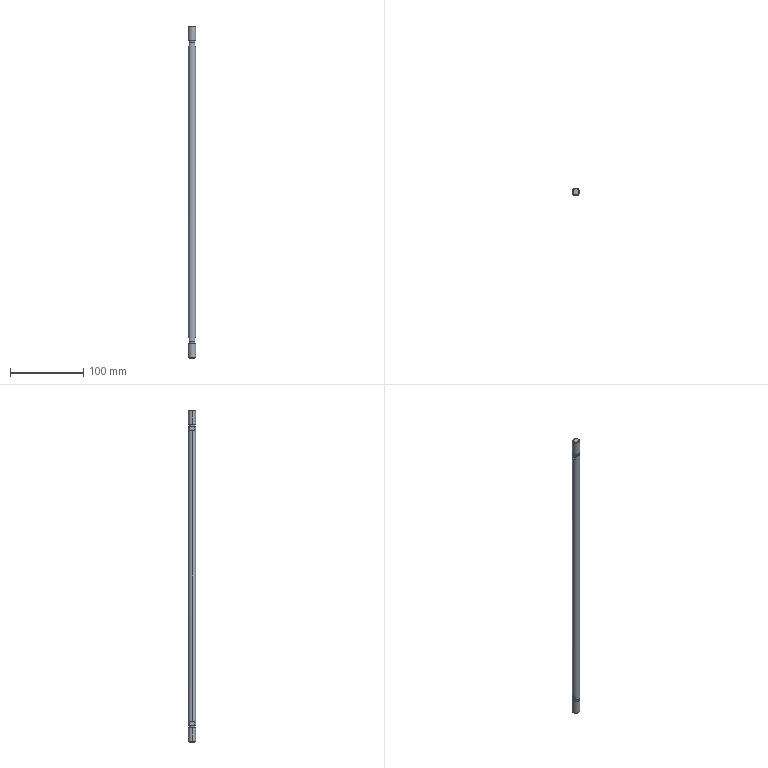Part | STEP file | rod_A_CDM2WB25_150_C76_0_ | 1 solid | 34 faces | box 10 x 10 x 452 mm | volume 35231 mm3 | plane 16 | cylinder 10 | cone 8 | commonest cylinder face diameters 10 x6 8.16 x4
STEP:
#1=CARTESIAN_POINT('',(4.08,0.,-420.));
#2=VERTEX_POINT('',#1);
#3=CARTESIAN_POINT('',(-4.08,0.,-420.));
#4=VERTEX_POINT('',#3);
#5=CARTESIAN_POINT('',(0.,0.,-420.));
#6=DIRECTION('',(0.,0.,1.));
#7=DIRECTION('',(1.,0.,0.));
#8=AXIS2_PLACEMENT_3D('',#5,#6,#7);
#9=CIRCLE('',#8,4.08);
#10=EDGE_CURVE('',#2,#4,#9,.T.);
#11=ORIENTED_EDGE('',*,*,#10,.T.);
#12=CARTESIAN_POINT('',(-5.,0.,-419.08));
#13=VERTEX_POINT('',#12);
#14=CARTESIAN_POINT('',(-4.08,0.,-420.));
#15=DIRECTION('',(-0.7071,0.,0.7071));
#16=VECTOR('',#15,1000.);
#17=LINE('',#14,#16);
#18=EDGE_CURVE('',#4,#13,#17,.T.);
#19=ORIENTED_EDGE('',*,*,#18,.T.);
#20=CARTESIAN_POINT('',(5.,0.,-419.08));
#21=VERTEX_POINT('',#20);
#22=CARTESIAN_POINT('',(0.,0.,-419.08));
#23=DIRECTION('',(0.,0.,1.));
#24=DIRECTION('',(1.,0.,0.));
#25=AXIS2_PLACEMENT_3D('',#22,#23,#24);
#26=CIRCLE('',#25,5.);
#27=EDGE_CURVE('',#21,#13,#26,.T.);
#28=ORIENTED_EDGE('',*,*,#27,.F.);
#29=CARTESIAN_POINT('',(4.08,0.,-420.));
#30=DIRECTION('',(0.7071,0.,0.7071));
#31=VECTOR('',#30,1000.);
#32=LINE('',#29,#31);
#33=EDGE_CURVE('',#2,#21,#32,.T.);
#34=ORIENTED_EDGE('',*,*,#33,.F.);
#35=EDGE_LOOP('',(#11,#19,#28,#34));
#36=FACE_OUTER_BOUND('',#35,.T.);
#37=CARTESIAN_POINT('',(0.,0.,-420.));
#38=DIRECTION('',(0.,0.,1.));
#39=DIRECTION('',(1.,0.,0.));
#40=AXIS2_PLACEMENT_3D('',#37,#38,#39);
#41=CONICAL_SURFACE('',#40,4.08,0.7854);
#42=ADVANCED_FACE('',(#36),#41,.T.);
#43=ORIENTED_EDGE('',*,*,#27,.T.);
#44=CARTESIAN_POINT('',(-5.,0.,-400.5));
#45=VERTEX_POINT('',#44);
#46=CARTESIAN_POINT('',(-5.,0.,-420.));
#47=DIRECTION('',(0.,0.,1.));
#48=VECTOR('',#47,1000.);
#49=LINE('',#46,#48);
#50=EDGE_CURVE('',#13,#45,#49,.T.);
#51=ORIENTED_EDGE('',*,*,#50,.T.);
#52=CARTESIAN_POINT('',(5.,0.,-400.5));
#53=VERTEX_POINT('',#52);
#54=CARTESIAN_POINT('',(0.,0.,-400.5));
#55=DIRECTION('',(0.,0.,1.));
#56=DIRECTION('',(1.,0.,0.));
#57=AXIS2_PLACEMENT_3D('',#54,#55,#56);
#58=CIRCLE('',#57,5.);
#59=EDGE_CURVE('',#53,#45,#58,.T.);
#60=ORIENTED_EDGE('',*,*,#59,.F.);
#61=CARTESIAN_POINT('',(5.,0.,-420.));
#62=DIRECTION('',(0.,0.,1.));
#63=VECTOR('',#62,1000.);
#64=LINE('',#61,#63);
#65=EDGE_CURVE('',#21,#53,#64,.T.);
#66=ORIENTED_EDGE('',*,*,#65,.F.);
#67=EDGE_LOOP('',(#43,#51,#60,#66));
#68=FACE_OUTER_BOUND('',#67,.T.);
#69=CARTESIAN_POINT('',(0.,0.,-420.));
#70=DIRECTION('',(0.,0.,1.));
#71=DIRECTION('',(1.,0.,0.));
#72=AXIS2_PLACEMENT_3D('',#69,#70,#71);
#73=CYLINDRICAL_SURFACE('',#72,5.);
#74=ADVANCED_FACE('',(#68),#73,.T.);
#75=CARTESIAN_POINT('',(4.08,0.,-400.5));
#76=VERTEX_POINT('',#75);
#77=CARTESIAN_POINT('',(-4.08,0.,-400.5));
#78=VERTEX_POINT('',#77);
#79=CARTESIAN_POINT('',(0.,0.,-400.5));
#80=DIRECTION('',(0.,0.,1.));
#81=DIRECTION('',(1.,0.,0.));
#82=AXIS2_PLACEMENT_3D('',#79,#80,#81);
#83=CIRCLE('',#82,4.08);
#84=EDGE_CURVE('',#76,#78,#83,.T.);
#85=ORIENTED_EDGE('',*,*,#84,.T.);
#86=CARTESIAN_POINT('',(-4.08,0.,-398.));
#87=VERTEX_POINT('',#86);
#88=CARTESIAN_POINT('',(-4.08,0.,-420.));
#89=DIRECTION('',(0.,0.,1.));
#90=VECTOR('',#89,1000.);
#91=LINE('',#88,#90);
#92=EDGE_CURVE('',#78,#87,#91,.T.);
#93=ORIENTED_EDGE('',*,*,#92,.T.);
#94=CARTESIAN_POINT('',(-4.,0.804,-398.));
#95=VERTEX_POINT('',#94);
#96=CARTESIAN_POINT('',(0.,0.,-398.));
#97=DIRECTION('',(0.,0.,1.));
#98=DIRECTION('',(1.,0.,0.));
#99=AXIS2_PLACEMENT_3D('',#96,#97,#98);
#100=CIRCLE('',#99,4.08);
#101=EDGE_CURVE('',#95,#87,#100,.T.);
#102=ORIENTED_EDGE('',*,*,#101,.F.);
#103=CARTESIAN_POINT('',(4.,0.804,-398.));
#104=VERTEX_POINT('',#103);
#105=CARTESIAN_POINT('',(0.,0.,-398.));
#106=DIRECTION('',(0.,0.,1.));
#107=DIRECTION('',(1.,0.,0.));
#108=AXIS2_PLACEMENT_3D('',#105,#106,#107);
#109=CIRCLE('',#108,4.08);
#110=EDGE_CURVE('',#104,#95,#109,.T.);
#111=ORIENTED_EDGE('',*,*,#110,.F.);
#112=CARTESIAN_POINT('',(4.08,0.,-398.));
#113=VERTEX_POINT('',#112);
#114=CARTESIAN_POINT('',(0.,0.,-398.));
#115=DIRECTION('',(0.,0.,1.));
#116=DIRECTION('',(1.,0.,0.));
#117=AXIS2_PLACEMENT_3D('',#114,#115,#116);
#118=CIRCLE('',#117,4.08);
#119=EDGE_CURVE('',#113,#104,#118,.T.);
#120=ORIENTED_EDGE('',*,*,#119,.F.);
#121=CARTESIAN_POINT('',(4.08,0.,-420.));
#122=DIRECTION('',(0.,0.,1.));
#123=VECTOR('',#122,1000.);
#124=LINE('',#121,#123);
#125=EDGE_CURVE('',#76,#113,#124,.T.);
#126=ORIENTED_EDGE('',*,*,#125,.F.);
#127=EDGE_LOOP('',(#85,#93,#102,#111,#120,#126));
#128=FACE_OUTER_BOUND('',#127,.T.);
#129=CARTESIAN_POINT('',(0.,0.,-420.));
#130=DIRECTION('',(0.,0.,1.));
#131=DIRECTION('',(1.,0.,0.));
#132=AXIS2_PLACEMENT_3D('',#129,#130,#131);
#133=CYLINDRICAL_SURFACE('',#132,4.08);
#134=ADVANCED_FACE('',(#128),#133,.T.);
#135=CARTESIAN_POINT('',(-4.,3.,-392.5));
#136=VERTEX_POINT('',#135);
#137=CARTESIAN_POINT('',(-5.,0.,-391.5));
#138=VERTEX_POINT('',#137);
#139=CARTESIAN_POINT('',(-4.,3.,-392.5));
#140=CARTESIAN_POINT('',(-4.655,2.127,-391.845));
#141=CARTESIAN_POINT('',(-5.,1.091,-391.5));
#142=CARTESIAN_POINT('',(-5.,0.,-391.5));
#143=(BOUNDED_CURVE()B_SPLINE_CURVE(3,(#139,#140,#141,#142),.UNSPECIFIED.,.F.,.T.)B_SPLINE_CURVE_WITH_KNOTS((4,4),(5.64,6.283),.UNSPECIFIED.)CURVE()GEOMETRIC_REPRESENTATION_ITEM()RATIONAL_B_SPLINE_CURVE((1.,0.9658,0.9658,1.))REPRESENTATION_ITEM(''));
#144=EDGE_CURVE('',#136,#138,#143,.T.);
#145=ORIENTED_EDGE('',*,*,#144,.T.);
#146=CARTESIAN_POINT('',(-5.,0.,3.5));
#147=VERTEX_POINT('',#146);
#148=CARTESIAN_POINT('',(-5.,0.,-420.));
#149=DIRECTION('',(0.,0.,1.));
#150=VECTOR('',#149,1000.);
#151=LINE('',#148,#150);
#152=EDGE_CURVE('',#138,#147,#151,.T.);
#153=ORIENTED_EDGE('',*,*,#152,.T.);
#154=CARTESIAN_POINT('',(-4.,3.,4.5));
#155=VERTEX_POINT('',#154);
#156=CARTESIAN_POINT('',(-5.,0.,3.5));
#157=CARTESIAN_POINT('',(-5.,1.091,3.5));
#158=CARTESIAN_POINT('',(-4.655,2.127,3.845));
#159=CARTESIAN_POINT('',(-4.,3.,4.5));
#160=(BOUNDED_CURVE()B_SPLINE_CURVE(3,(#156,#157,#158,#159),.UNSPECIFIED.,.F.,.T.)B_SPLINE_CURVE_WITH_KNOTS((4,4),(3.142,3.785),.UNSPECIFIED.)CURVE()GEOMETRIC_REPRESENTATION_ITEM()RATIONAL_B_SPLINE_CURVE((1.,0.9658,0.9658,1.))REPRESENTATION_ITEM(''));
#161=EDGE_CURVE('',#147,#155,#160,.T.);
#162=ORIENTED_EDGE('',*,*,#161,.T.);
#163=CARTESIAN_POINT('',(-4.,3.,9.08));
#164=VERTEX_POINT('',#163);
#165=CARTESIAN_POINT('',(-4.,3.,-420.));
#166=DIRECTION('',(0.,0.,1.));
#167=VECTOR('',#166,1000.);
#168=LINE('',#165,#167);
#169=EDGE_CURVE('',#155,#164,#168,.T.);
#170=ORIENTED_EDGE('',*,*,#169,.T.);
#171=CARTESIAN_POINT('',(4.,3.,9.08));
#172=VERTEX_POINT('',#171);
#173=CARTESIAN_POINT('',(0.,0.,9.08));
#174=DIRECTION('',(0.,0.,1.));
#175=DIRECTION('',(1.,0.,0.));
#176=AXIS2_PLACEMENT_3D('',#173,#174,#175);
#177=CIRCLE('',#176,5.);
#178=EDGE_CURVE('',#172,#164,#177,.T.);
#179=ORIENTED_EDGE('',*,*,#178,.F.);
#180=CARTESIAN_POINT('',(4.,3.,4.5));
#181=VERTEX_POINT('',#180);
#182=CARTESIAN_POINT('',(4.,3.,-420.));
#183=DIRECTION('',(0.,0.,-1.));
#184=VECTOR('',#183,1000.);
#185=LINE('',#182,#184);
#186=EDGE_CURVE('',#172,#181,#185,.T.);
#187=ORIENTED_EDGE('',*,*,#186,.T.);
#188=CARTESIAN_POINT('',(5.,0.,3.5));
#189=VERTEX_POINT('',#188);
#190=CARTESIAN_POINT('',(4.,3.,4.5));
#191=CARTESIAN_POINT('',(4.655,2.127,3.845));
#192=CARTESIAN_POINT('',(5.,1.091,3.5));
#193=CARTESIAN_POINT('',(5.,0.,3.5));
#194=(BOUNDED_CURVE()B_SPLINE_CURVE(3,(#190,#191,#192,#193),.UNSPECIFIED.,.F.,.T.)B_SPLINE_CURVE_WITH_KNOTS((4,4),(2.498,3.142),.UNSPECIFIED.)CURVE()GEOMETRIC_REPRESENTATION_ITEM()RATIONAL_B_SPLINE_CURVE((1.,0.9658,0.9658,1.))REPRESENTATION_ITEM(''));
#195=EDGE_CURVE('',#181,#189,#194,.T.);
#196=ORIENTED_EDGE('',*,*,#195,.T.);
#197=CARTESIAN_POINT('',(5.,0.,-391.5));
#198=VERTEX_POINT('',#197);
#199=CARTESIAN_POINT('',(5.,0.,-420.));
#200=DIRECTION('',(0.,0.,1.));
#201=VECTOR('',#200,1000.);
#202=LINE('',#199,#201);
#203=EDGE_CURVE('',#198,#189,#202,.T.);
#204=ORIENTED_EDGE('',*,*,#203,.F.);
#205=CARTESIAN_POINT('',(4.,3.,-392.5));
#206=VERTEX_POINT('',#205);
#207=CARTESIAN_POINT('',(5.,0.,-391.5));
#208=CARTESIAN_POINT('',(5.,1.091,-391.5));
#209=CARTESIAN_POINT('',(4.655,2.127,-391.845));
#210=CARTESIAN_POINT('',(4.,3.,-392.5));
#211=(BOUNDED_CURVE()B_SPLINE_CURVE(3,(#207,#208,#209,#210),.UNSPECIFIED.,.F.,.T.)B_SPLINE_CURVE_WITH_KNOTS((4,4),(0.,0.6435),.UNSPECIFIED.)CURVE()GEOMETRIC_REPRESENTATION_ITEM()RATIONAL_B_SPLINE_CURVE((1.,0.9658,0.9658,1.))REPRESENTATION_ITEM(''));
#212=EDGE_CURVE('',#198,#206,#211,.T.);
#213=ORIENTED_EDGE('',*,*,#212,.T.);
#214=CARTESIAN_POINT('',(4.,3.,-397.08));
#215=VERTEX_POINT('',#214);
#216=CARTESIAN_POINT('',(4.,3.,-420.));
#217=DIRECTION('',(0.,0.,-1.));
#218=VECTOR('',#217,1000.);
#219=LINE('',#216,#218);
#220=EDGE_CURVE('',#206,#215,#219,.T.);
#221=ORIENTED_EDGE('',*,*,#220,.T.);
#222=CARTESIAN_POINT('',(-4.,3.,-397.08));
#223=VERTEX_POINT('',#222);
#224=CARTESIAN_POINT('',(0.,0.,-397.08));
#225=DIRECTION('',(0.,0.,1.));
#226=DIRECTION('',(1.,0.,0.));
#227=AXIS2_PLACEMENT_3D('',#224,#225,#226);
#228=CIRCLE('',#227,5.);
#229=EDGE_CURVE('',#215,#223,#228,.T.);
#230=ORIENTED_EDGE('',*,*,#229,.T.);
#231=CARTESIAN_POINT('',(-4.,3.,-420.));
#232=DIRECTION('',(0.,0.,1.));
#233=VECTOR('',#232,1000.);
#234=LINE('',#231,#233);
#235=EDGE_CURVE('',#223,#136,#234,.T.);
#236=ORIENTED_EDGE('',*,*,#235,.T.);
#237=EDGE_LOOP('',(#145,#153,#162,#170,#179,#187,#196,#204,#213,#221,#230,#236));
#238=FACE_OUTER_BOUND('',#237,.T.);
#239=CARTESIAN_POINT('',(0.,0.,-420.));
#240=DIRECTION('',(0.,0.,1.));
#241=DIRECTION('',(1.,0.,0.));
#242=AXIS2_PLACEMENT_3D('',#239,#240,#241);
#243=CYLINDRICAL_SURFACE('',#242,5.);
#244=ADVANCED_FACE('',(#238),#243,.T.);
#245=CARTESIAN_POINT('',(-4.,0.804,10.));
#246=VERTEX_POINT('',#245);
#247=CARTESIAN_POINT('',(-4.08,0.,10.));
#248=VERTEX_POINT('',#247);
#249=CARTESIAN_POINT('',(0.,0.,10.));
#250=DIRECTION('',(0.,0.,1.));
#251=DIRECTION('',(1.,0.,0.));
#252=AXIS2_PLACEMENT_3D('',#249,#250,#251);
#253=CIRCLE('',#252,4.08);
#254=EDGE_CURVE('',#246,#248,#253,.T.);
#255=ORIENTED_EDGE('',*,*,#254,.T.);
#256=CARTESIAN_POINT('',(-4.08,0.,12.5));
#257=VERTEX_POINT('',#256);
#258=CARTESIAN_POINT('',(-4.08,0.,-420.));
#259=DIRECTION('',(0.,0.,1.));
#260=VECTOR('',#259,1000.);
#261=LINE('',#258,#260);
#262=EDGE_CURVE('',#248,#257,#261,.T.);
#263=ORIENTED_EDGE('',*,*,#262,.T.);
#264=CARTESIAN_POINT('',(4.08,0.,12.5));
#265=VERTEX_POINT('',#264);
#266=CARTESIAN_POINT('',(0.,0.,12.5));
#267=DIRECTION('',(0.,0.,1.));
#268=DIRECTION('',(1.,0.,0.));
#269=AXIS2_PLACEMENT_3D('',#266,#267,#268);
#270=CIRCLE('',#269,4.08);
#271=EDGE_CURVE('',#265,#257,#270,.T.);
#272=ORIENTED_EDGE('',*,*,#271,.F.);
#273=CARTESIAN_POINT('',(4.08,0.,10.));
#274=VERTEX_POINT('',#273);
#275=CARTESIAN_POINT('',(4.08,0.,-420.));
#276=DIRECTION('',(0.,0.,1.));
#277=VECTOR('',#276,1000.);
#278=LINE('',#275,#277);
#279=EDGE_CURVE('',#274,#265,#278,.T.);
#280=ORIENTED_EDGE('',*,*,#279,.F.);
#281=CARTESIAN_POINT('',(4.,0.804,10.));
#282=VERTEX_POINT('',#281);
#283=CARTESIAN_POINT('',(0.,0.,10.));
#284=DIRECTION('',(0.,0.,1.));
#285=DIRECTION('',(1.,0.,0.));
#286=AXIS2_PLACEMENT_3D('',#283,#284,#285);
#287=CIRCLE('',#286,4.08);
#288=EDGE_CURVE('',#274,#282,#287,.T.);
#289=ORIENTED_EDGE('',*,*,#288,.T.);
#290=CARTESIAN_POINT('',(0.,0.,10.));
#291=DIRECTION('',(0.,0.,1.));
#292=DIRECTION('',(1.,0.,0.));
#293=AXIS2_PLACEMENT_3D('',#290,#291,#292);
#294=CIRCLE('',#293,4.08);
#295=EDGE_CURVE('',#282,#246,#294,.T.);
#296=ORIENTED_EDGE('',*,*,#295,.T.);
#297=EDGE_LOOP('',(#255,#263,#272,#280,#289,#296));
#298=FACE_OUTER_BOUND('',#297,.T.);
#299=CARTESIAN_POINT('',(0.,0.,-420.));
#300=DIRECTION('',(0.,0.,1.));
#301=DIRECTION('',(1.,0.,0.));
#302=AXIS2_PLACEMENT_3D('',#299,#300,#301);
#303=CYLINDRICAL_SURFACE('',#302,4.08);
#304=ADVANCED_FACE('',(#298),#303,.T.);
#305=CARTESIAN_POINT('',(5.,0.,12.5));
#306=VERTEX_POINT('',#305);
#307=CARTESIAN_POINT('',(-5.,0.,12.5));
#308=VERTEX_POINT('',#307);
#309=CARTESIAN_POINT('',(0.,0.,12.5));
#310=DIRECTION('',(0.,0.,1.));
#311=DIRECTION('',(1.,0.,0.));
#312=AXIS2_PLACEMENT_3D('',#309,#310,#311);
#313=CIRCLE('',#312,5.);
#314=EDGE_CURVE('',#306,#308,#313,.T.);
#315=ORIENTED_EDGE('',*,*,#314,.T.);
#316=CARTESIAN_POINT('',(-5.,0.,31.08));
#317=VERTEX_POINT('',#316);
#318=CARTESIAN_POINT('',(-5.,0.,-420.));
#319=DIRECTION('',(0.,0.,1.));
#320=VECTOR('',#319,1000.);
#321=LINE('',#318,#320);
#322=EDGE_CURVE('',#308,#317,#321,.T.);
#323=ORIENTED_EDGE('',*,*,#322,.T.);
#324=CARTESIAN_POINT('',(5.,0.,31.08));
#325=VERTEX_POINT('',#324);
#326=CARTESIAN_POINT('',(0.,0.,31.08));
#327=DIRECTION('',(0.,0.,1.));
#328=DIRECTION('',(1.,0.,0.));
#329=AXIS2_PLACEMENT_3D('',#326,#327,#328);
#330=CIRCLE('',#329,5.);
#331=EDGE_CURVE('',#325,#317,#330,.T.);
#332=ORIENTED_EDGE('',*,*,#331,.F.);
#333=CARTESIAN_POINT('',(5.,0.,-420.));
#334=DIRECTION('',(0.,0.,1.));
#335=VECTOR('',#334,1000.);
#336=LINE('',#333,#335);
#337=EDGE_CURVE('',#306,#325,#336,.T.);
#338=ORIENTED_EDGE('',*,*,#337,.F.);
#339=EDGE_LOOP('',(#315,#323,#332,#338));
#340=FACE_OUTER_BOUND('',#339,.T.);
#341=CARTESIAN_POINT('',(0.,0.,-420.));
#342=DIRECTION('',(0.,0.,1.));
#343=DIRECTION('',(1.,0.,0.));
#344=AXIS2_PLACEMENT_3D('',#341,#342,#343);
#345=CYLINDRICAL_SURFACE('',#344,5.);
#346=ADVANCED_FACE('',(#340),#345,.T.);
#347=CARTESIAN_POINT('',(4.08,0.,32.));
#348=VERTEX_POINT('',#347);
#349=CARTESIAN_POINT('',(-4.08,0.,32.));
#350=VERTEX_POINT('',#349);
#351=CARTESIAN_POINT('',(0.,0.,32.));
#352=DIRECTION('',(0.,0.,1.));
#353=DIRECTION('',(1.,0.,0.));
#354=AXIS2_PLACEMENT_3D('',#351,#352,#353);
#355=CIRCLE('',#354,4.08);
#356=EDGE_CURVE('',#348,#350,#355,.T.);
#357=ORIENTED_EDGE('',*,*,#356,.F.);
#358=CARTESIAN_POINT('',(5.,0.,31.08));
#359=DIRECTION('',(0.7071,0.,-0.7071));
#360=VECTOR('',#359,1000.);
#361=LINE('',#358,#360);
#362=EDGE_CURVE('',#348,#325,#361,.T.);
#363=ORIENTED_EDGE('',*,*,#362,.T.);
#364=ORIENTED_EDGE('',*,*,#331,.T.);
#365=CARTESIAN_POINT('',(-5.,0.,31.08));
#366=DIRECTION('',(-0.7071,0.,-0.7071));
#367=VECTOR('',#366,1000.);
#368=LINE('',#365,#367);
#369=EDGE_CURVE('',#350,#317,#368,.T.);
#370=ORIENTED_EDGE('',*,*,#369,.F.);
#371=EDGE_LOOP('',(#357,#363,#364,#370));
#372=FACE_OUTER_BOUND('',#371,.T.);
#373=CARTESIAN_POINT('',(0.,0.,31.08));
#374=DIRECTION('',(0.,0.,-1.));
#375=DIRECTION('',(-1.,0.,0.));
#376=AXIS2_PLACEMENT_3D('',#373,#374,#375);
#377=CONICAL_SURFACE('',#376,5.,0.7854);
#378=ADVANCED_FACE('',(#372),#377,.T.);
#379=CARTESIAN_POINT('',(-4.,-3.,-397.08));
#380=VERTEX_POINT('',#379);
#381=CARTESIAN_POINT('',(4.,-3.,-397.08));
#382=VERTEX_POINT('',#381);
#383=CARTESIAN_POINT('',(0.,0.,-397.08));
#384=DIRECTION('',(0.,0.,1.));
#385=DIRECTION('',(1.,0.,0.));
#386=AXIS2_PLACEMENT_3D('',#383,#384,#385);
#387=CIRCLE('',#386,5.);
#388=EDGE_CURVE('',#380,#382,#387,.T.);
#389=ORIENTED_EDGE('',*,*,#388,.F.);
#390=CARTESIAN_POINT('',(-4.,-0.804,-398.));
#391=VERTEX_POINT('',#390);
#392=CARTESIAN_POINT('',(-4.,-3.,-397.08));
#393=CARTESIAN_POINT('',(-4.,-2.657,-397.286));
#394=CARTESIAN_POINT('',(-4.,-2.306,-397.474));
#395=CARTESIAN_POINT('',(-4.,-1.576,-397.793));
#396=CARTESIAN_POINT('',(-4.,-1.193,-397.923));
#397=CARTESIAN_POINT('',(-4.,-0.804,-398.));
#398=B_SPLINE_CURVE_WITH_KNOTS('',3,(#392,#393,#394,#395,#396,#397),.UNSPECIFIED.,.F.,.F.,(4,2,4),(0.00946,0.01066,0.01185),.UNSPECIFIED.);
#399=EDGE_CURVE('',#380,#391,#398,.T.);
#400=ORIENTED_EDGE('',*,*,#399,.T.);
#401=CARTESIAN_POINT('',(4.,-0.804,-398.));
#402=VERTEX_POINT('',#401);
#403=CARTESIAN_POINT('',(0.,0.,-398.));
#404=DIRECTION('',(0.,0.,1.));
#405=DIRECTION('',(1.,0.,0.));
#406=AXIS2_PLACEMENT_3D('',#403,#404,#405);
#407=CIRCLE('',#406,4.08);
#408=EDGE_CURVE('',#391,#402,#407,.T.);
#409=ORIENTED_EDGE('',*,*,#408,.T.);
#410=CARTESIAN_POINT('',(4.,-0.804,-398.));
#411=CARTESIAN_POINT('',(4.,-1.195,-397.923));
#412=CARTESIAN_POINT('',(4.,-1.58,-397.792));
#413=CARTESIAN_POINT('',(4.,-2.311,-397.472));
#414=CARTESIAN_POINT('',(4.,-2.66,-397.284));
#415=CARTESIAN_POINT('',(4.,-3.,-397.08));
#416=B_SPLINE_CURVE_WITH_KNOTS('',3,(#410,#411,#412,#413,#414,#415),.UNSPECIFIED.,.F.,.F.,(4,2,4),(0.01347,0.01467,0.01588),.UNSPECIFIED.);
#417=EDGE_CURVE('',#402,#382,#416,.T.);
#418=ORIENTED_EDGE('',*,*,#417,.T.);
#419=EDGE_LOOP('',(#389,#400,#409,#418));
#420=FACE_OUTER_BOUND('',#419,.T.);
#421=CARTESIAN_POINT('',(0.,0.,-398.));
#422=DIRECTION('',(0.,0.,1.));
#423=DIRECTION('',(1.,0.,0.));
#424=AXIS2_PLACEMENT_3D('',#421,#422,#423);
#425=CONICAL_SURFACE('',#424,4.08,0.7854);
#426=ADVANCED_FACE('',(#420),#425,.T.);
#427=ORIENTED_EDGE('',*,*,#178,.T.);
#428=CARTESIAN_POINT('',(-4.,3.,9.08));
#429=CARTESIAN_POINT('',(-4.,2.657,9.286));
#430=CARTESIAN_POINT('',(-4.,2.306,9.474));
#431=CARTESIAN_POINT('',(-4.,1.576,9.793));
#432=CARTESIAN_POINT('',(-4.,1.193,9.923));
#433=CARTESIAN_POINT('',(-4.,0.804,10.));
#434=B_SPLINE_CURVE_WITH_KNOTS('',3,(#428,#429,#430,#431,#432,#433),.UNSPECIFIED.,.F.,.F.,(4,2,4),(0.00946,0.01066,0.01185),.UNSPECIFIED.);
#435=EDGE_CURVE('',#164,#246,#434,.T.);
#436=ORIENTED_EDGE('',*,*,#435,.T.);
#437=ORIENTED_EDGE('',*,*,#295,.F.);
#438=CARTESIAN_POINT('',(4.,0.804,10.));
#439=CARTESIAN_POINT('',(4.,1.195,9.923));
#440=CARTESIAN_POINT('',(4.,1.58,9.792));
#441=CARTESIAN_POINT('',(4.,2.311,9.472));
#442=CARTESIAN_POINT('',(4.,2.66,9.284));
#443=CARTESIAN_POINT('',(4.,3.,9.08));
#444=B_SPLINE_CURVE_WITH_KNOTS('',3,(#438,#439,#440,#441,#442,#443),.UNSPECIFIED.,.F.,.F.,(4,2,4),(0.01347,0.01467,0.01588),.UNSPECIFIED.);
#445=EDGE_CURVE('',#282,#172,#444,.T.);
#446=ORIENTED_EDGE('',*,*,#445,.T.);
#447=EDGE_LOOP('',(#427,#436,#437,#446));
#448=FACE_OUTER_BOUND('',#447,.T.);
#449=CARTESIAN_POINT('',(0.,0.,9.08));
#450=DIRECTION('',(0.,0.,-1.));
#451=DIRECTION('',(-1.,0.,0.));
#452=AXIS2_PLACEMENT_3D('',#449,#450,#451);
#453=CONICAL_SURFACE('',#452,5.,0.7854);
#454=ADVANCED_FACE('',(#448),#453,.T.);
#455=CARTESIAN_POINT('',(0.,0.,32.));
#456=DIRECTION('',(0.,0.,1.));
#457=DIRECTION('',(1.,0.,0.));
#458=AXIS2_PLACEMENT_3D('',#455,#456,#457);
#459=CIRCLE('',#458,4.08);
#460=EDGE_CURVE('',#350,#348,#459,.T.);
#461=ORIENTED_EDGE('',*,*,#460,.T.);
#462=ORIENTED_EDGE('',*,*,#356,.T.);
#463=EDGE_LOOP('',(#461,#462));
#464=FACE_OUTER_BOUND('',#463,.T.);
#465=CARTESIAN_POINT('',(0.,0.,32.));
#466=DIRECTION('',(0.,0.,-1.));
#467=DIRECTION('',(-1.,0.,0.));
#468=AXIS2_PLACEMENT_3D('',#465,#466,#467);
#469=PLANE('',#468);
#470=ADVANCED_FACE('',(#464),#469,.F.);
#471=ORIENTED_EDGE('',*,*,#362,.F.);
#472=ORIENTED_EDGE('',*,*,#460,.F.);
#473=ORIENTED_EDGE('',*,*,#369,.T.);
#474=CARTESIAN_POINT('',(0.,0.,31.08));
#475=DIRECTION('',(0.,0.,1.));
#476=DIRECTION('',(1.,0.,0.));
#477=AXIS2_PLACEMENT_3D('',#474,#475,#476);
#478=CIRCLE('',#477,5.);
#479=EDGE_CURVE('',#317,#325,#478,.T.);
#480=ORIENTED_EDGE('',*,*,#479,.T.);
#481=EDGE_LOOP('',(#471,#472,#473,#480));
#482=FACE_OUTER_BOUND('',#481,.T.);
#483=CARTESIAN_POINT('',(0.,0.,31.08));
#484=DIRECTION('',(0.,0.,-1.));
#485=DIRECTION('',(-1.,0.,0.));
#486=AXIS2_PLACEMENT_3D('',#483,#484,#485);
#487=CONICAL_SURFACE('',#486,5.,0.7854);
#488=ADVANCED_FACE('',(#482),#487,.T.);
#489=ORIENTED_EDGE('',*,*,#322,.F.);
#490=CARTESIAN_POINT('',(0.,0.,12.5));
#491=DIRECTION('',(0.,0.,1.));
#492=DIRECTION('',(1.,0.,0.));
#493=AXIS2_PLACEMENT_3D('',#490,#491,#492);
#494=CIRCLE('',#493,5.);
#495=EDGE_CURVE('',#308,#306,#494,.T.);
#496=ORIENTED_EDGE('',*,*,#495,.T.);
#497=ORIENTED_EDGE('',*,*,#337,.T.);
#498=ORIENTED_EDGE('',*,*,#479,.F.);
#499=EDGE_LOOP('',(#489,#496,#497,#498));
#500=FACE_OUTER_BOUND('',#499,.T.);
#501=CARTESIAN_POINT('',(0.,0.,-420.));
#502=DIRECTION('',(0.,0.,1.));
#503=DIRECTION('',(1.,0.,0.));
#504=AXIS2_PLACEMENT_3D('',#501,#502,#503);
#505=CYLINDRICAL_SURFACE('',#504,5.);
#506=ADVANCED_FACE('',(#500),#505,.T.);
#507=ORIENTED_EDGE('',*,*,#314,.F.);
#508=ORIENTED_EDGE('',*,*,#495,.F.);
#509=EDGE_LOOP('',(#507,#508));
#510=FACE_OUTER_BOUND('',#509,.T.);
#511=ORIENTED_EDGE('',*,*,#271,.T.);
#512=CARTESIAN_POINT('',(0.,0.,12.5));
#513=DIRECTION('',(0.,0.,1.));
#514=DIRECTION('',(1.,0.,0.));
#515=AXIS2_PLACEMENT_3D('',#512,#513,#514);
#516=CIRCLE('',#515,4.08);
#517=EDGE_CURVE('',#257,#265,#516,.T.);
#518=ORIENTED_EDGE('',*,*,#517,.T.);
#519=EDGE_LOOP('',(#511,#518));
#520=FACE_BOUND('',#519,.T.);
#521=CARTESIAN_POINT('',(0.,5.,12.5));
#522=DIRECTION('',(0.,0.,1.));
#523=DIRECTION('',(1.,0.,0.));
#524=AXIS2_PLACEMENT_3D('',#521,#522,#523);
#525=PLANE('',#524);
#526=ADVANCED_FACE('',(#510,#520),#525,.F.);
#527=ORIENTED_EDGE('',*,*,#262,.F.);
#528=CARTESIAN_POINT('',(-4.,-0.804,10.));
#529=VERTEX_POINT('',#528);
#530=CARTESIAN_POINT('',(0.,0.,10.));
#531=DIRECTION('',(0.,0.,1.));
#532=DIRECTION('',(1.,0.,0.));
#533=AXIS2_PLACEMENT_3D('',#530,#531,#532);
#534=CIRCLE('',#533,4.08);
#535=EDGE_CURVE('',#248,#529,#534,.T.);
#536=ORIENTED_EDGE('',*,*,#535,.T.);
#537=CARTESIAN_POINT('',(4.,-0.804,10.));
#538=VERTEX_POINT('',#537);
#539=CARTESIAN_POINT('',(0.,0.,10.));
#540=DIRECTION('',(0.,0.,1.));
#541=DIRECTION('',(1.,0.,0.));
#542=AXIS2_PLACEMENT_3D('',#539,#540,#541);
#543=CIRCLE('',#542,4.08);
#544=EDGE_CURVE('',#529,#538,#543,.T.);
#545=ORIENTED_EDGE('',*,*,#544,.T.);
#546=CARTESIAN_POINT('',(0.,0.,10.));
#547=DIRECTION('',(0.,0.,1.));
#548=DIRECTION('',(1.,0.,0.));
#549=AXIS2_PLACEMENT_3D('',#546,#547,#548);
#550=CIRCLE('',#549,4.08);
#551=EDGE_CURVE('',#538,#274,#550,.T.);
#552=ORIENTED_EDGE('',*,*,#551,.T.);
#553=ORIENTED_EDGE('',*,*,#279,.T.);
#554=ORIENTED_EDGE('',*,*,#517,.F.);
#555=EDGE_LOOP('',(#527,#536,#545,#552,#553,#554));
#556=FACE_OUTER_BOUND('',#555,.T.);
#557=CARTESIAN_POINT('',(0.,0.,-420.));
#558=DIRECTION('',(0.,0.,1.));
#559=DIRECTION('',(1.,0.,0.));
#560=AXIS2_PLACEMENT_3D('',#557,#558,#559);
#561=CYLINDRICAL_SURFACE('',#560,4.08);
#562=ADVANCED_FACE('',(#556),#561,.T.);
#563=ORIENTED_EDGE('',*,*,#544,.F.);
#564=CARTESIAN_POINT('',(-4.,-3.,9.08));
#565=VERTEX_POINT('',#564);
#566=CARTESIAN_POINT('',(-4.,-0.804,10.));
#567=CARTESIAN_POINT('',(-4.,-1.195,9.923));
#568=CARTESIAN_POINT('',(-4.,-1.58,9.792));
#569=CARTESIAN_POINT('',(-4.,-2.311,9.472));
#570=CARTESIAN_POINT('',(-4.,-2.66,9.284));
#571=CARTESIAN_POINT('',(-4.,-3.,9.08));
#572=B_SPLINE_CURVE_WITH_KNOTS('',3,(#566,#567,#568,#569,#570,#571),.UNSPECIFIED.,.F.,.F.,(4,2,4),(0.01347,0.01467,0.01588),.UNSPECIFIED.);
#573=EDGE_CURVE('',#529,#565,#572,.T.);
#574=ORIENTED_EDGE('',*,*,#573,.T.);
#575=CARTESIAN_POINT('',(4.,-3.,9.08));
#576=VERTEX_POINT('',#575);
#577=CARTESIAN_POINT('',(0.,0.,9.08));
#578=DIRECTION('',(0.,0.,1.));
#579=DIRECTION('',(1.,0.,0.));
#580=AXIS2_PLACEMENT_3D('',#577,#578,#579);
#581=CIRCLE('',#580,5.);
#582=EDGE_CURVE('',#565,#576,#581,.T.);
#583=ORIENTED_EDGE('',*,*,#582,.T.);
#584=CARTESIAN_POINT('',(4.,-3.,9.08));
#585=CARTESIAN_POINT('',(4.,-2.657,9.286));
#586=CARTESIAN_POINT('',(4.,-2.306,9.474));
#587=CARTESIAN_POINT('',(4.,-1.576,9.793));
#588=CARTESIAN_POINT('',(4.,-1.193,9.923));
#589=CARTESIAN_POINT('',(4.,-0.804,10.));
#590=B_SPLINE_CURVE_WITH_KNOTS('',3,(#584,#585,#586,#587,#588,#589),.UNSPECIFIED.,.F.,.F.,(4,2,4),(0.00946,0.01066,0.01185),.UNSPECIFIED.);
#591=EDGE_CURVE('',#576,#538,#590,.T.);
#592=ORIENTED_EDGE('',*,*,#591,.T.);
#593=EDGE_LOOP('',(#563,#574,#583,#592));
#594=FACE_OUTER_BOUND('',#593,.T.);
#595=CARTESIAN_POINT('',(0.,0.,9.08));
#596=DIRECTION('',(0.,0.,-1.));
#597=DIRECTION('',(-1.,0.,0.));
#598=AXIS2_PLACEMENT_3D('',#595,#596,#597);
#599=CONICAL_SURFACE('',#598,5.,0.7854);
#600=ADVANCED_FACE('',(#594),#599,.T.);
#601=ORIENTED_EDGE('',*,*,#152,.F.);
#602=CARTESIAN_POINT('',(-4.,-3.,-392.5));
#603=VERTEX_POINT('',#602);
#604=CARTESIAN_POINT('',(-5.,0.,-391.5));
#605=CARTESIAN_POINT('',(-5.,-1.091,-391.5));
#606=CARTESIAN_POINT('',(-4.655,-2.127,-391.845));
#607=CARTESIAN_POINT('',(-4.,-3.,-392.5));
#608=(BOUNDED_CURVE()B_SPLINE_CURVE(3,(#604,#605,#606,#607),.UNSPECIFIED.,.F.,.F.)B_SPLINE_CURVE_WITH_KNOTS((4,4),(0.,0.6435),.UNSPECIFIED.)CURVE()GEOMETRIC_REPRESENTATION_ITEM()RATIONAL_B_SPLINE_CURVE((1.,0.9658,0.9658,1.))REPRESENTATION_ITEM(''));
#609=EDGE_CURVE('',#138,#603,#608,.T.);
#610=ORIENTED_EDGE('',*,*,#609,.T.);
#611=CARTESIAN_POINT('',(-4.,-3.,-420.));
#612=DIRECTION('',(0.,0.,-1.));
#613=VECTOR('',#612,1000.);
#614=LINE('',#611,#613);
#615=EDGE_CURVE('',#603,#380,#614,.T.);
#616=ORIENTED_EDGE('',*,*,#615,.T.);
#617=ORIENTED_EDGE('',*,*,#388,.T.);
#618=CARTESIAN_POINT('',(4.,-3.,-392.5));
#619=VERTEX_POINT('',#618);
#620=CARTESIAN_POINT('',(4.,-3.,-420.));
#621=DIRECTION('',(0.,0.,1.));
#622=VECTOR('',#621,1000.);
#623=LINE('',#620,#622);
#624=EDGE_CURVE('',#382,#619,#623,.T.);
#625=ORIENTED_EDGE('',*,*,#624,.T.);
#626=CARTESIAN_POINT('',(4.,-3.,-392.5));
#627=CARTESIAN_POINT('',(4.655,-2.127,-391.845));
#628=CARTESIAN_POINT('',(5.,-1.091,-391.5));
#629=CARTESIAN_POINT('',(5.,0.,-391.5));
#630=(BOUNDED_CURVE()B_SPLINE_CURVE(3,(#626,#627,#628,#629),.UNSPECIFIED.,.F.,.F.)B_SPLINE_CURVE_WITH_KNOTS((4,4),(5.64,6.283),.UNSPECIFIED.)CURVE()GEOMETRIC_REPRESENTATION_ITEM()RATIONAL_B_SPLINE_CURVE((1.,0.9658,0.9658,1.))REPRESENTATION_ITEM(''));
#631=EDGE_CURVE('',#619,#198,#630,.T.);
#632=ORIENTED_EDGE('',*,*,#631,.T.);
#633=ORIENTED_EDGE('',*,*,#203,.T.);
#634=CARTESIAN_POINT('',(4.,-3.,4.5));
#635=VERTEX_POINT('',#634);
#636=CARTESIAN_POINT('',(5.,0.,3.5));
#637=CARTESIAN_POINT('',(5.,-1.091,3.5));
#638=CARTESIAN_POINT('',(4.655,-2.127,3.845));
#639=CARTESIAN_POINT('',(4.,-3.,4.5));
#640=(BOUNDED_CURVE()B_SPLINE_CURVE(3,(#636,#637,#638,#639),.UNSPECIFIED.,.F.,.F.)B_SPLINE_CURVE_WITH_KNOTS((4,4),(3.142,3.785),.UNSPECIFIED.)CURVE()GEOMETRIC_REPRESENTATION_ITEM()RATIONAL_B_SPLINE_CURVE((1.,0.9658,0.9658,1.))REPRESENTATION_ITEM(''));
#641=EDGE_CURVE('',#189,#635,#640,.T.);
#642=ORIENTED_EDGE('',*,*,#641,.T.);
#643=CARTESIAN_POINT('',(4.,-3.,-420.));
#644=DIRECTION('',(0.,0.,1.));
#645=VECTOR('',#644,1000.);
#646=LINE('',#643,#645);
#647=EDGE_CURVE('',#635,#576,#646,.T.);
#648=ORIENTED_EDGE('',*,*,#647,.T.);
#649=ORIENTED_EDGE('',*,*,#582,.F.);
#650=CARTESIAN_POINT('',(-4.,-3.,4.5));
#651=VERTEX_POINT('',#650);
#652=CARTESIAN_POINT('',(-4.,-3.,-420.));
#653=DIRECTION('',(0.,0.,-1.));
#654=VECTOR('',#653,1000.);
#655=LINE('',#652,#654);
#656=EDGE_CURVE('',#565,#651,#655,.T.);
#657=ORIENTED_EDGE('',*,*,#656,.T.);
#658=CARTESIAN_POINT('',(-4.,-3.,4.5));
#659=CARTESIAN_POINT('',(-4.655,-2.127,3.845));
#660=CARTESIAN_POINT('',(-5.,-1.091,3.5));
#661=CARTESIAN_POINT('',(-5.,0.,3.5));
#662=(BOUNDED_CURVE()B_SPLINE_CURVE(3,(#658,#659,#660,#661),.UNSPECIFIED.,.F.,.F.)B_SPLINE_CURVE_WITH_KNOTS((4,4),(2.498,3.142),.UNSPECIFIED.)CURVE()GEOMETRIC_REPRESENTATION_ITEM()RATIONAL_B_SPLINE_CURVE((1.,0.9658,0.9658,1.))REPRESENTATION_ITEM(''));
#663=EDGE_CURVE('',#651,#147,#662,.T.);
#664=ORIENTED_EDGE('',*,*,#663,.T.);
#665=EDGE_LOOP('',(#601,#610,#616,#617,#625,#632,#633,#642,#648,#649,#657,#664));
#666=FACE_OUTER_BOUND('',#665,.T.);
#667=CARTESIAN_POINT('',(0.,0.,-420.));
#668=DIRECTION('',(0.,0.,1.));
#669=DIRECTION('',(1.,0.,0.));
#670=AXIS2_PLACEMENT_3D('',#667,#668,#669);
#671=CYLINDRICAL_SURFACE('',#670,5.);
#672=ADVANCED_FACE('',(#666),#671,.T.);
#673=ORIENTED_EDGE('',*,*,#110,.T.);
#674=CARTESIAN_POINT('',(-4.,0.804,-398.));
#675=CARTESIAN_POINT('',(-4.,1.195,-397.923));
#676=CARTESIAN_POINT('',(-4.,1.58,-397.792));
#677=CARTESIAN_POINT('',(-4.,2.311,-397.472));
#678=CARTESIAN_POINT('',(-4.,2.66,-397.284));
#679=CARTESIAN_POINT('',(-4.,3.,-397.08));
#680=B_SPLINE_CURVE_WITH_KNOTS('',3,(#674,#675,#676,#677,#678,#679),.UNSPECIFIED.,.F.,.F.,(4,2,4),(0.01347,0.01467,0.01588),.UNSPECIFIED.);
#681=EDGE_CURVE('',#95,#223,#680,.T.);
#682=ORIENTED_EDGE('',*,*,#681,.T.);
#683=ORIENTED_EDGE('',*,*,#229,.F.);
#684=CARTESIAN_POINT('',(4.,3.,-397.08));
#685=CARTESIAN_POINT('',(4.,2.657,-397.286));
#686=CARTESIAN_POINT('',(4.,2.306,-397.474));
#687=CARTESIAN_POINT('',(4.,1.576,-397.793));
#688=CARTESIAN_POINT('',(4.,1.193,-397.923));
#689=CARTESIAN_POINT('',(4.,0.804,-398.));
#690=B_SPLINE_CURVE_WITH_KNOTS('',3,(#684,#685,#686,#687,#688,#689),.UNSPECIFIED.,.F.,.F.,(4,2,4),(0.00946,0.01066,0.01185),.UNSPECIFIED.);
#691=EDGE_CURVE('',#215,#104,#690,.T.);
#692=ORIENTED_EDGE('',*,*,#691,.T.);
#693=EDGE_LOOP('',(#673,#682,#683,#692));
#694=FACE_OUTER_BOUND('',#693,.T.);
#695=CARTESIAN_POINT('',(0.,0.,-398.));
#696=DIRECTION('',(0.,0.,1.));
#697=DIRECTION('',(1.,0.,0.));
#698=AXIS2_PLACEMENT_3D('',#695,#696,#697);
#699=CONICAL_SURFACE('',#698,4.08,0.7854);
#700=ADVANCED_FACE('',(#694),#699,.T.);
#701=ORIENTED_EDGE('',*,*,#92,.F.);
#702=CARTESIAN_POINT('',(0.,0.,-400.5));
#703=DIRECTION('',(0.,0.,1.));
#704=DIRECTION('',(1.,0.,0.));
#705=AXIS2_PLACEMENT_3D('',#702,#703,#704);
#706=CIRCLE('',#705,4.08);
#707=EDGE_CURVE('',#78,#76,#706,.T.);
#708=ORIENTED_EDGE('',*,*,#707,.T.);
#709=ORIENTED_EDGE('',*,*,#125,.T.);
#710=CARTESIAN_POINT('',(0.,0.,-398.));
#711=DIRECTION('',(0.,0.,1.));
#712=DIRECTION('',(1.,0.,0.));
#713=AXIS2_PLACEMENT_3D('',#710,#711,#712);
#714=CIRCLE('',#713,4.08);
#715=EDGE_CURVE('',#402,#113,#714,.T.);
#716=ORIENTED_EDGE('',*,*,#715,.F.);
#717=ORIENTED_EDGE('',*,*,#408,.F.);
#718=CARTESIAN_POINT('',(0.,0.,-398.));
#719=DIRECTION('',(0.,0.,1.));
#720=DIRECTION('',(1.,0.,0.));
#721=AXIS2_PLACEMENT_3D('',#718,#719,#720);
#722=CIRCLE('',#721,4.08);
#723=EDGE_CURVE('',#87,#391,#722,.T.);
#724=ORIENTED_EDGE('',*,*,#723,.F.);
#725=EDGE_LOOP('',(#701,#708,#709,#716,#717,#724));
#726=FACE_OUTER_BOUND('',#725,.T.);
#727=CARTESIAN_POINT('',(0.,0.,-420.));
#728=DIRECTION('',(0.,0.,1.));
#729=DIRECTION('',(1.,0.,0.));
#730=AXIS2_PLACEMENT_3D('',#727,#728,#729);
#731=CYLINDRICAL_SURFACE('',#730,4.08);
#732=ADVANCED_FACE('',(#726),#731,.T.);
#733=ORIENTED_EDGE('',*,*,#84,.F.);
#734=ORIENTED_EDGE('',*,*,#707,.F.);
#735=EDGE_LOOP('',(#733,#734));
#736=FACE_BOUND('',#735,.T.);
#737=ORIENTED_EDGE('',*,*,#59,.T.);
#738=CARTESIAN_POINT('',(0.,0.,-400.5));
#739=DIRECTION('',(0.,0.,1.));
#740=DIRECTION('',(1.,0.,0.));
#741=AXIS2_PLACEMENT_3D('',#738,#739,#740);
#742=CIRCLE('',#741,5.);
#743=EDGE_CURVE('',#45,#53,#742,.T.);
#744=ORIENTED_EDGE('',*,*,#743,.T.);
#745=EDGE_LOOP('',(#737,#744));
#746=FACE_OUTER_BOUND('',#745,.T.);
#747=CARTESIAN_POINT('',(0.,4.08,-400.5));
#748=DIRECTION('',(0.,0.,-1.));
#749=DIRECTION('',(-1.,0.,0.));
#750=AXIS2_PLACEMENT_3D('',#747,#748,#749);
#751=PLANE('',#750);
#752=ADVANCED_FACE('',(#736,#746),#751,.F.);
#753=ORIENTED_EDGE('',*,*,#50,.F.);
#754=CARTESIAN_POINT('',(0.,0.,-419.08));
#755=DIRECTION('',(0.,0.,1.));
#756=DIRECTION('',(1.,0.,0.));
#757=AXIS2_PLACEMENT_3D('',#754,#755,#756);
#758=CIRCLE('',#757,5.);
#759=EDGE_CURVE('',#13,#21,#758,.T.);
#760=ORIENTED_EDGE('',*,*,#759,.T.);
#761=ORIENTED_EDGE('',*,*,#65,.T.);
#762=ORIENTED_EDGE('',*,*,#743,.F.);
#763=EDGE_LOOP('',(#753,#760,#761,#762));
#764=FACE_OUTER_BOUND('',#763,.T.);
#765=CARTESIAN_POINT('',(0.,0.,-420.));
#766=DIRECTION('',(0.,0.,1.));
#767=DIRECTION('',(1.,0.,0.));
#768=AXIS2_PLACEMENT_3D('',#765,#766,#767);
#769=CYLINDRICAL_SURFACE('',#768,5.);
#770=ADVANCED_FACE('',(#764),#769,.T.);
#771=ORIENTED_EDGE('',*,*,#18,.F.);
#772=CARTESIAN_POINT('',(0.,0.,-420.));
#773=DIRECTION('',(0.,0.,1.));
#774=DIRECTION('',(1.,0.,0.));
#775=AXIS2_PLACEMENT_3D('',#772,#773,#774);
#776=CIRCLE('',#775,4.08);
#777=EDGE_CURVE('',#4,#2,#776,.T.);
#778=ORIENTED_EDGE('',*,*,#777,.T.);
#779=ORIENTED_EDGE('',*,*,#33,.T.);
#780=ORIENTED_EDGE('',*,*,#759,.F.);
#781=EDGE_LOOP('',(#771,#778,#779,#780));
#782=FACE_OUTER_BOUND('',#781,.T.);
#783=CARTESIAN_POINT('',(0.,0.,-420.));
#784=DIRECTION('',(0.,0.,1.));
#785=DIRECTION('',(1.,0.,0.));
#786=AXIS2_PLACEMENT_3D('',#783,#784,#785);
#787=CONICAL_SURFACE('',#786,4.08,0.7854);
#788=ADVANCED_FACE('',(#782),#787,.T.);
#789=ORIENTED_EDGE('',*,*,#10,.F.);
#790=ORIENTED_EDGE('',*,*,#777,.F.);
#791=EDGE_LOOP('',(#789,#790));
#792=FACE_OUTER_BOUND('',#791,.T.);
#793=CARTESIAN_POINT('',(0.,4.08,-420.));
#794=DIRECTION('',(0.,0.,1.));
#795=DIRECTION('',(1.,0.,0.));
#796=AXIS2_PLACEMENT_3D('',#793,#794,#795);
#797=PLANE('',#796);
#798=ADVANCED_FACE('',(#792),#797,.F.);
#799=CARTESIAN_POINT('',(4.,-10.,10.));
#800=DIRECTION('',(0.,1.,0.));
#801=VECTOR('',#800,1000.);
#802=LINE('',#799,#801);
#803=EDGE_CURVE('',#538,#282,#802,.T.);
#804=ORIENTED_EDGE('',*,*,#803,.T.);
#805=ORIENTED_EDGE('',*,*,#288,.F.);
#806=ORIENTED_EDGE('',*,*,#551,.F.);
#807=EDGE_LOOP('',(#804,#805,#806));
#808=FACE_OUTER_BOUND('',#807,.T.);
#809=CARTESIAN_POINT('',(4.,-10.,10.));
#810=DIRECTION('',(0.,0.,1.));
#811=DIRECTION('',(1.,0.,0.));
#812=AXIS2_PLACEMENT_3D('',#809,#810,#811);
#813=PLANE('',#812);
#814=ADVANCED_FACE('',(#808),#813,.F.);
#815=ORIENTED_EDGE('',*,*,#647,.F.);
#816=CARTESIAN_POINT('',(4.,-10.,4.5));
#817=DIRECTION('',(0.,1.,0.));
#818=VECTOR('',#817,1000.);
#819=LINE('',#816,#818);
#820=EDGE_CURVE('',#635,#181,#819,.T.);
#821=ORIENTED_EDGE('',*,*,#820,.T.);
#822=ORIENTED_EDGE('',*,*,#186,.F.);
#823=ORIENTED_EDGE('',*,*,#445,.F.);
#824=ORIENTED_EDGE('',*,*,#803,.F.);
#825=ORIENTED_EDGE('',*,*,#591,.F.);
#826=EDGE_LOOP('',(#815,#821,#822,#823,#824,#825));
#827=FACE_OUTER_BOUND('',#826,.T.);
#828=CARTESIAN_POINT('',(4.,-10.,4.5));
#829=DIRECTION('',(-1.,0.,0.));
#830=DIRECTION('',(0.,0.,1.));
#831=AXIS2_PLACEMENT_3D('',#828,#829,#830);
#832=PLANE('',#831);
#833=ADVANCED_FACE('',(#827),#832,.F.);
#834=ORIENTED_EDGE('',*,*,#820,.F.);
#835=ORIENTED_EDGE('',*,*,#641,.F.);
#836=ORIENTED_EDGE('',*,*,#195,.F.);
#837=EDGE_LOOP('',(#834,#835,#836));
#838=FACE_OUTER_BOUND('',#837,.T.);
#839=CARTESIAN_POINT('',(5.,-10.,3.5));
#840=DIRECTION('',(-0.7071,0.,-0.7071));
#841=DIRECTION('',(-0.7071,0.,0.7071));
#842=AXIS2_PLACEMENT_3D('',#839,#840,#841);
#843=PLANE('',#842);
#844=ADVANCED_FACE('',(#838),#843,.F.);
#845=CARTESIAN_POINT('',(-4.,-10.,10.));
#846=DIRECTION('',(0.,1.,0.));
#847=VECTOR('',#846,1000.);
#848=LINE('',#845,#847);
#849=EDGE_CURVE('',#529,#246,#848,.T.);
#850=ORIENTED_EDGE('',*,*,#849,.F.);
#851=ORIENTED_EDGE('',*,*,#535,.F.);
#852=ORIENTED_EDGE('',*,*,#254,.F.);
#853=EDGE_LOOP('',(#850,#851,#852));
#854=FACE_OUTER_BOUND('',#853,.T.);
#855=CARTESIAN_POINT('',(-7.,-10.,10.));
#856=DIRECTION('',(0.,0.,1.));
#857=DIRECTION('',(1.,0.,0.));
#858=AXIS2_PLACEMENT_3D('',#855,#856,#857);
#859=PLANE('',#858);
#860=ADVANCED_FACE('',(#854),#859,.F.);
#861=CARTESIAN_POINT('',(-4.,-10.,4.5));
#862=DIRECTION('',(0.,1.,0.));
#863=VECTOR('',#862,1000.);
#864=LINE('',#861,#863);
#865=EDGE_CURVE('',#651,#155,#864,.T.);
#866=ORIENTED_EDGE('',*,*,#865,.T.);
#867=ORIENTED_EDGE('',*,*,#161,.F.);
#868=ORIENTED_EDGE('',*,*,#663,.F.);
#869=EDGE_LOOP('',(#866,#867,#868));
#870=FACE_OUTER_BOUND('',#869,.T.);
#871=CARTESIAN_POINT('',(-4.,-10.,4.5));
#872=DIRECTION('',(0.7071,0.,-0.7071));
#873=DIRECTION('',(-0.7071,0.,-0.7071));
#874=AXIS2_PLACEMENT_3D('',#871,#872,#873);
#875=PLANE('',#874);
#876=ADVANCED_FACE('',(#870),#875,.F.);
#877=ORIENTED_EDGE('',*,*,#169,.F.);
#878=ORIENTED_EDGE('',*,*,#865,.F.);
#879=ORIENTED_EDGE('',*,*,#656,.F.);
#880=ORIENTED_EDGE('',*,*,#573,.F.);
#881=ORIENTED_EDGE('',*,*,#849,.T.);
#882=ORIENTED_EDGE('',*,*,#435,.F.);
#883=EDGE_LOOP('',(#877,#878,#879,#880,#881,#882));
#884=FACE_OUTER_BOUND('',#883,.T.);
#885=CARTESIAN_POINT('',(-4.,-10.,10.));
#886=DIRECTION('',(1.,0.,0.));
#887=DIRECTION('',(0.,0.,-1.));
#888=AXIS2_PLACEMENT_3D('',#885,#886,#887);
#889=PLANE('',#888);
#890=ADVANCED_FACE('',(#884),#889,.F.);
#891=ORIENTED_EDGE('',*,*,#631,.F.);
#892=CARTESIAN_POINT('',(4.,-10.,-392.5));
#893=DIRECTION('',(0.,1.,0.));
#894=VECTOR('',#893,1000.);
#895=LINE('',#892,#894);
#896=EDGE_CURVE('',#619,#206,#895,.T.);
#897=ORIENTED_EDGE('',*,*,#896,.T.);
#898=ORIENTED_EDGE('',*,*,#212,.F.);
#899=EDGE_LOOP('',(#891,#897,#898));
#900=FACE_OUTER_BOUND('',#899,.T.);
#901=CARTESIAN_POINT('',(4.,-10.,-392.5));
#902=DIRECTION('',(-0.7071,0.,0.7071));
#903=DIRECTION('',(0.7071,0.,0.7071));
#904=AXIS2_PLACEMENT_3D('',#901,#902,#903);
#905=PLANE('',#904);
#906=ADVANCED_FACE('',(#900),#905,.F.);
#907=ORIENTED_EDGE('',*,*,#896,.F.);
#908=ORIENTED_EDGE('',*,*,#624,.F.);
#909=ORIENTED_EDGE('',*,*,#417,.F.);
#910=CARTESIAN_POINT('',(4.,-10.,-398.));
#911=DIRECTION('',(0.,1.,0.));
#912=VECTOR('',#911,1000.);
#913=LINE('',#910,#912);
#914=EDGE_CURVE('',#402,#104,#913,.T.);
#915=ORIENTED_EDGE('',*,*,#914,.T.);
#916=ORIENTED_EDGE('',*,*,#691,.F.);
#917=ORIENTED_EDGE('',*,*,#220,.F.);
#918=EDGE_LOOP('',(#907,#908,#909,#915,#916,#917));
#919=FACE_OUTER_BOUND('',#918,.T.);
#920=CARTESIAN_POINT('',(4.,-10.,-398.));
#921=DIRECTION('',(-1.,0.,0.));
#922=DIRECTION('',(0.,0.,1.));
#923=AXIS2_PLACEMENT_3D('',#920,#921,#922);
#924=PLANE('',#923);
#925=ADVANCED_FACE('',(#919),#924,.F.);
#926=ORIENTED_EDGE('',*,*,#914,.F.);
#927=ORIENTED_EDGE('',*,*,#715,.T.);
#928=ORIENTED_EDGE('',*,*,#119,.T.);
#929=EDGE_LOOP('',(#926,#927,#928));
#930=FACE_OUTER_BOUND('',#929,.T.);
#931=CARTESIAN_POINT('',(7.,-10.,-398.));
#932=DIRECTION('',(0.,0.,-1.));
#933=DIRECTION('',(-1.,0.,0.));
#934=AXIS2_PLACEMENT_3D('',#931,#932,#933);
#935=PLANE('',#934);
#936=ADVANCED_FACE('',(#930),#935,.F.);
#937=ORIENTED_EDGE('',*,*,#144,.F.);
#938=CARTESIAN_POINT('',(-4.,-10.,-392.5));
#939=DIRECTION('',(0.,1.,0.));
#940=VECTOR('',#939,1000.);
#941=LINE('',#938,#940);
#942=EDGE_CURVE('',#603,#136,#941,.T.);
#943=ORIENTED_EDGE('',*,*,#942,.F.);
#944=ORIENTED_EDGE('',*,*,#609,.F.);
#945=EDGE_LOOP('',(#937,#943,#944));
#946=FACE_OUTER_BOUND('',#945,.T.);
#947=CARTESIAN_POINT('',(-5.,-10.,-391.5));
#948=DIRECTION('',(0.7071,0.,0.7071));
#949=DIRECTION('',(0.7071,0.,-0.7071));
#950=AXIS2_PLACEMENT_3D('',#947,#948,#949);
#951=PLANE('',#950);
#952=ADVANCED_FACE('',(#946),#951,.F.);
#953=ORIENTED_EDGE('',*,*,#942,.T.);
#954=ORIENTED_EDGE('',*,*,#235,.F.);
#955=ORIENTED_EDGE('',*,*,#681,.F.);
#956=CARTESIAN_POINT('',(-4.,-10.,-398.));
#957=DIRECTION('',(0.,1.,0.));
#958=VECTOR('',#957,1000.);
#959=LINE('',#956,#958);
#960=EDGE_CURVE('',#391,#95,#959,.T.);
#961=ORIENTED_EDGE('',*,*,#960,.F.);
#962=ORIENTED_EDGE('',*,*,#399,.F.);
#963=ORIENTED_EDGE('',*,*,#615,.F.);
#964=EDGE_LOOP('',(#953,#954,#955,#961,#962,#963));
#965=FACE_OUTER_BOUND('',#964,.T.);
#966=CARTESIAN_POINT('',(-4.,-10.,-392.5));
#967=DIRECTION('',(1.,0.,0.));
#968=DIRECTION('',(0.,0.,-1.));
#969=AXIS2_PLACEMENT_3D('',#966,#967,#968);
#970=PLANE('',#969);
#971=ADVANCED_FACE('',(#965),#970,.F.);
#972=ORIENTED_EDGE('',*,*,#960,.T.);
#973=ORIENTED_EDGE('',*,*,#101,.T.);
#974=ORIENTED_EDGE('',*,*,#723,.T.);
#975=EDGE_LOOP('',(#972,#973,#974));
#976=FACE_OUTER_BOUND('',#975,.T.);
#977=CARTESIAN_POINT('',(-4.,-10.,-398.));
#978=DIRECTION('',(0.,0.,-1.));
#979=DIRECTION('',(-1.,0.,0.));
#980=AXIS2_PLACEMENT_3D('',#977,#978,#979);
#981=PLANE('',#980);
#982=ADVANCED_FACE('',(#976),#981,.F.);
#983=CLOSED_SHELL('',(#42,#74,#134,#244,#304,#346,#378,#426,#454,#470,#488,#506,#526,#562,#600,#672,#700,#732,#752,#770,#788,#798,#814,#833,#844,#860,#876,#890,#906,#925,#936,#952,#971,#982));
#984=MANIFOLD_SOLID_BREP('',#983);
#985=CARTESIAN_POINT('',(0.,0.,0.));
#986=DIRECTION('',(0.,0.,1.));
#987=DIRECTION('',(1.,0.,0.));
#988=AXIS2_PLACEMENT_3D('',#985,#986,#987);
#989=(LENGTH_UNIT()NAMED_UNIT(*)SI_UNIT(.MILLI.,.METRE.));
#990=UNCERTAINTY_MEASURE_WITH_UNIT(LENGTH_MEASURE(0.00001),#989,'','');
#991=(NAMED_UNIT(*)PLANE_ANGLE_UNIT()SI_UNIT($,.RADIAN.));
#992=(NAMED_UNIT(*)SI_UNIT($,.STERADIAN.)SOLID_ANGLE_UNIT());
#993=(GEOMETRIC_REPRESENTATION_CONTEXT(3)GLOBAL_UNCERTAINTY_ASSIGNED_CONTEXT((#990))GLOBAL_UNIT_ASSIGNED_CONTEXT((#989,#991,#992))REPRESENTATION_CONTEXT('',''));
#994=ADVANCED_BREP_SHAPE_REPRESENTATION('',(#984,#988),#993);